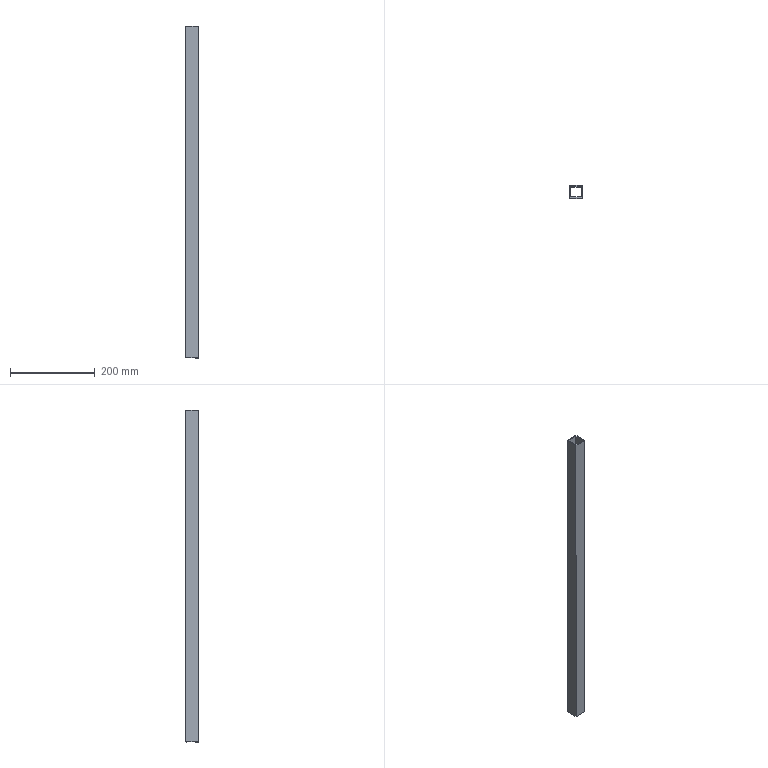Part | SolidWorks | features Extrusion 1 | 1 solid | 10 faces | box 30 x 30 x 784 mm | volume 254016 mm3 | plane 10
STEP:
#1=CARTESIAN_POINT('',(-16.115,15.846,784.));
#2=VERTEX_POINT('',#1);
#3=CARTESIAN_POINT('',(-16.115,-14.154,784.));
#4=VERTEX_POINT('',#3);
#5=CARTESIAN_POINT('',(-16.115,-14.154,784.));
#6=DIRECTION('',(0.,-1.,0.));
#7=VECTOR('',#6,1000.);
#8=LINE('',#5,#7);
#9=EDGE_CURVE('',#2,#4,#8,.T.);
#10=ORIENTED_EDGE('',*,*,#9,.T.);
#11=CARTESIAN_POINT('',(13.885,-14.154,784.));
#12=VERTEX_POINT('',#11);
#13=CARTESIAN_POINT('',(13.885,-14.154,784.));
#14=DIRECTION('',(1.,0.,0.));
#15=VECTOR('',#14,1000.);
#16=LINE('',#13,#15);
#17=EDGE_CURVE('',#4,#12,#16,.T.);
#18=ORIENTED_EDGE('',*,*,#17,.T.);
#19=CARTESIAN_POINT('',(13.885,15.846,784.));
#20=VERTEX_POINT('',#19);
#21=CARTESIAN_POINT('',(13.885,15.846,784.));
#22=DIRECTION('',(0.,1.,0.));
#23=VECTOR('',#22,1000.);
#24=LINE('',#21,#23);
#25=EDGE_CURVE('',#12,#20,#24,.T.);
#26=ORIENTED_EDGE('',*,*,#25,.T.);
#27=CARTESIAN_POINT('',(-16.115,15.846,784.));
#28=DIRECTION('',(-1.,0.,0.));
#29=VECTOR('',#28,1000.);
#30=LINE('',#27,#29);
#31=EDGE_CURVE('',#20,#2,#30,.T.);
#32=ORIENTED_EDGE('',*,*,#31,.T.);
#33=EDGE_LOOP('',(#10,#18,#26,#32));
#34=FACE_OUTER_BOUND('',#33,.T.);
#35=CARTESIAN_POINT('',(-13.115,12.846,784.));
#36=VERTEX_POINT('',#35);
#37=CARTESIAN_POINT('',(-13.115,-11.154,784.));
#38=VERTEX_POINT('',#37);
#39=CARTESIAN_POINT('',(-13.115,-11.154,784.));
#40=DIRECTION('',(0.,-1.,0.));
#41=VECTOR('',#40,1000.);
#42=LINE('',#39,#41);
#43=EDGE_CURVE('',#36,#38,#42,.T.);
#44=ORIENTED_EDGE('',*,*,#43,.F.);
#45=CARTESIAN_POINT('',(10.885,12.846,784.));
#46=VERTEX_POINT('',#45);
#47=CARTESIAN_POINT('',(-13.115,12.846,784.));
#48=DIRECTION('',(-1.,0.,0.));
#49=VECTOR('',#48,1000.);
#50=LINE('',#47,#49);
#51=EDGE_CURVE('',#46,#36,#50,.T.);
#52=ORIENTED_EDGE('',*,*,#51,.F.);
#53=CARTESIAN_POINT('',(10.885,-11.154,784.));
#54=VERTEX_POINT('',#53);
#55=CARTESIAN_POINT('',(10.885,12.846,784.));
#56=DIRECTION('',(0.,1.,0.));
#57=VECTOR('',#56,1000.);
#58=LINE('',#55,#57);
#59=EDGE_CURVE('',#54,#46,#58,.T.);
#60=ORIENTED_EDGE('',*,*,#59,.F.);
#61=CARTESIAN_POINT('',(10.885,-11.154,784.));
#62=DIRECTION('',(1.,0.,0.));
#63=VECTOR('',#62,1000.);
#64=LINE('',#61,#63);
#65=EDGE_CURVE('',#38,#54,#64,.T.);
#66=ORIENTED_EDGE('',*,*,#65,.F.);
#67=EDGE_LOOP('',(#44,#52,#60,#66));
#68=FACE_BOUND('',#67,.T.);
#69=CARTESIAN_POINT('',(-0.000000003,0.000000004,784.));
#70=DIRECTION('',(0.,0.,-1.));
#71=DIRECTION('',(-1.,0.,0.));
#72=AXIS2_PLACEMENT_3D('',#69,#70,#71);
#73=PLANE('',#72);
#74=ADVANCED_FACE('',(#34,#68),#73,.F.);
#75=CARTESIAN_POINT('',(-16.115,15.846,0.000000013));
#76=VERTEX_POINT('',#75);
#77=CARTESIAN_POINT('',(-16.115,-14.154,0.000000013));
#78=VERTEX_POINT('',#77);
#79=CARTESIAN_POINT('',(-16.115,-14.154,0.000000013));
#80=DIRECTION('',(0.,-1.,0.));
#81=VECTOR('',#80,1000.);
#82=LINE('',#79,#81);
#83=EDGE_CURVE('',#76,#78,#82,.T.);
#84=ORIENTED_EDGE('',*,*,#83,.F.);
#85=CARTESIAN_POINT('',(13.885,15.846,0.000000013));
#86=VERTEX_POINT('',#85);
#87=CARTESIAN_POINT('',(-16.115,15.846,0.000000013));
#88=DIRECTION('',(-1.,0.,0.));
#89=VECTOR('',#88,1000.);
#90=LINE('',#87,#89);
#91=EDGE_CURVE('',#86,#76,#90,.T.);
#92=ORIENTED_EDGE('',*,*,#91,.F.);
#93=CARTESIAN_POINT('',(13.885,-14.154,0.000000013));
#94=VERTEX_POINT('',#93);
#95=CARTESIAN_POINT('',(13.885,15.846,0.000000013));
#96=DIRECTION('',(0.,1.,0.));
#97=VECTOR('',#96,1000.);
#98=LINE('',#95,#97);
#99=EDGE_CURVE('',#94,#86,#98,.T.);
#100=ORIENTED_EDGE('',*,*,#99,.F.);
#101=CARTESIAN_POINT('',(13.885,-14.154,0.000000013));
#102=DIRECTION('',(1.,0.,0.));
#103=VECTOR('',#102,1000.);
#104=LINE('',#101,#103);
#105=EDGE_CURVE('',#78,#94,#104,.T.);
#106=ORIENTED_EDGE('',*,*,#105,.F.);
#107=EDGE_LOOP('',(#84,#92,#100,#106));
#108=FACE_OUTER_BOUND('',#107,.T.);
#109=CARTESIAN_POINT('',(10.885,12.846,0.000000013));
#110=VERTEX_POINT('',#109);
#111=CARTESIAN_POINT('',(-13.115,12.846,0.000000013));
#112=VERTEX_POINT('',#111);
#113=CARTESIAN_POINT('',(-13.115,12.846,0.000000013));
#114=DIRECTION('',(-1.,0.,0.));
#115=VECTOR('',#114,1000.);
#116=LINE('',#113,#115);
#117=EDGE_CURVE('',#110,#112,#116,.T.);
#118=ORIENTED_EDGE('',*,*,#117,.T.);
#119=CARTESIAN_POINT('',(-13.115,-11.154,0.000000013));
#120=VERTEX_POINT('',#119);
#121=CARTESIAN_POINT('',(-13.115,-11.154,0.000000013));
#122=DIRECTION('',(0.,-1.,0.));
#123=VECTOR('',#122,1000.);
#124=LINE('',#121,#123);
#125=EDGE_CURVE('',#112,#120,#124,.T.);
#126=ORIENTED_EDGE('',*,*,#125,.T.);
#127=CARTESIAN_POINT('',(10.885,-11.154,0.000000013));
#128=VERTEX_POINT('',#127);
#129=CARTESIAN_POINT('',(10.885,-11.154,0.000000013));
#130=DIRECTION('',(1.,0.,0.));
#131=VECTOR('',#130,1000.);
#132=LINE('',#129,#131);
#133=EDGE_CURVE('',#120,#128,#132,.T.);
#134=ORIENTED_EDGE('',*,*,#133,.T.);
#135=CARTESIAN_POINT('',(10.885,12.846,0.000000013));
#136=DIRECTION('',(0.,1.,0.));
#137=VECTOR('',#136,1000.);
#138=LINE('',#135,#137);
#139=EDGE_CURVE('',#128,#110,#138,.T.);
#140=ORIENTED_EDGE('',*,*,#139,.T.);
#141=EDGE_LOOP('',(#118,#126,#134,#140));
#142=FACE_BOUND('',#141,.T.);
#143=CARTESIAN_POINT('',(-0.000000003,0.000000004,0.000000013));
#144=DIRECTION('',(0.,0.,-1.));
#145=DIRECTION('',(-1.,0.,0.));
#146=AXIS2_PLACEMENT_3D('',#143,#144,#145);
#147=PLANE('',#146);
#148=ADVANCED_FACE('',(#108,#142),#147,.T.);
#149=ORIENTED_EDGE('',*,*,#83,.T.);
#150=CARTESIAN_POINT('',(-16.115,-14.154,784.));
#151=DIRECTION('',(0.,0.,-1.));
#152=VECTOR('',#151,1000.);
#153=LINE('',#150,#152);
#154=EDGE_CURVE('',#4,#78,#153,.T.);
#155=ORIENTED_EDGE('',*,*,#154,.F.);
#156=ORIENTED_EDGE('',*,*,#9,.F.);
#157=CARTESIAN_POINT('',(-16.115,15.846,784.));
#158=DIRECTION('',(0.,0.,-1.));
#159=VECTOR('',#158,1000.);
#160=LINE('',#157,#159);
#161=EDGE_CURVE('',#2,#76,#160,.T.);
#162=ORIENTED_EDGE('',*,*,#161,.T.);
#163=EDGE_LOOP('',(#149,#155,#156,#162));
#164=FACE_OUTER_BOUND('',#163,.T.);
#165=CARTESIAN_POINT('',(-16.115,-14.154,784.));
#166=DIRECTION('',(1.,0.,0.));
#167=DIRECTION('',(0.,0.,-1.));
#168=AXIS2_PLACEMENT_3D('',#165,#166,#167);
#169=PLANE('',#168);
#170=ADVANCED_FACE('',(#164),#169,.F.);
#171=ORIENTED_EDGE('',*,*,#105,.T.);
#172=CARTESIAN_POINT('',(13.885,-14.154,784.));
#173=DIRECTION('',(0.,0.,-1.));
#174=VECTOR('',#173,1000.);
#175=LINE('',#172,#174);
#176=EDGE_CURVE('',#12,#94,#175,.T.);
#177=ORIENTED_EDGE('',*,*,#176,.F.);
#178=ORIENTED_EDGE('',*,*,#17,.F.);
#179=ORIENTED_EDGE('',*,*,#154,.T.);
#180=EDGE_LOOP('',(#171,#177,#178,#179));
#181=FACE_OUTER_BOUND('',#180,.T.);
#182=CARTESIAN_POINT('',(13.885,-14.154,784.));
#183=DIRECTION('',(0.,1.,0.));
#184=DIRECTION('',(-1.,0.,0.));
#185=AXIS2_PLACEMENT_3D('',#182,#183,#184);
#186=PLANE('',#185);
#187=ADVANCED_FACE('',(#181),#186,.F.);
#188=ORIENTED_EDGE('',*,*,#99,.T.);
#189=CARTESIAN_POINT('',(13.885,15.846,784.));
#190=DIRECTION('',(0.,0.,-1.));
#191=VECTOR('',#190,1000.);
#192=LINE('',#189,#191);
#193=EDGE_CURVE('',#20,#86,#192,.T.);
#194=ORIENTED_EDGE('',*,*,#193,.F.);
#195=ORIENTED_EDGE('',*,*,#25,.F.);
#196=ORIENTED_EDGE('',*,*,#176,.T.);
#197=EDGE_LOOP('',(#188,#194,#195,#196));
#198=FACE_OUTER_BOUND('',#197,.T.);
#199=CARTESIAN_POINT('',(13.885,15.846,784.));
#200=DIRECTION('',(-1.,0.,0.));
#201=DIRECTION('',(0.,-1.,0.));
#202=AXIS2_PLACEMENT_3D('',#199,#200,#201);
#203=PLANE('',#202);
#204=ADVANCED_FACE('',(#198),#203,.F.);
#205=ORIENTED_EDGE('',*,*,#91,.T.);
#206=ORIENTED_EDGE('',*,*,#161,.F.);
#207=ORIENTED_EDGE('',*,*,#31,.F.);
#208=ORIENTED_EDGE('',*,*,#193,.T.);
#209=EDGE_LOOP('',(#205,#206,#207,#208));
#210=FACE_OUTER_BOUND('',#209,.T.);
#211=CARTESIAN_POINT('',(-16.115,15.846,784.));
#212=DIRECTION('',(0.,-1.,0.));
#213=DIRECTION('',(0.,0.,-1.));
#214=AXIS2_PLACEMENT_3D('',#211,#212,#213);
#215=PLANE('',#214);
#216=ADVANCED_FACE('',(#210),#215,.F.);
#217=ORIENTED_EDGE('',*,*,#125,.F.);
#218=CARTESIAN_POINT('',(-13.115,12.846,784.));
#219=DIRECTION('',(0.,0.,-1.));
#220=VECTOR('',#219,1000.);
#221=LINE('',#218,#220);
#222=EDGE_CURVE('',#36,#112,#221,.T.);
#223=ORIENTED_EDGE('',*,*,#222,.F.);
#224=ORIENTED_EDGE('',*,*,#43,.T.);
#225=CARTESIAN_POINT('',(-13.115,-11.154,784.));
#226=DIRECTION('',(0.,0.,-1.));
#227=VECTOR('',#226,1000.);
#228=LINE('',#225,#227);
#229=EDGE_CURVE('',#38,#120,#228,.T.);
#230=ORIENTED_EDGE('',*,*,#229,.T.);
#231=EDGE_LOOP('',(#217,#223,#224,#230));
#232=FACE_OUTER_BOUND('',#231,.T.);
#233=CARTESIAN_POINT('',(-13.115,-11.154,784.));
#234=DIRECTION('',(1.,0.,0.));
#235=DIRECTION('',(0.,1.,0.));
#236=AXIS2_PLACEMENT_3D('',#233,#234,#235);
#237=PLANE('',#236);
#238=ADVANCED_FACE('',(#232),#237,.T.);
#239=ORIENTED_EDGE('',*,*,#133,.F.);
#240=ORIENTED_EDGE('',*,*,#229,.F.);
#241=ORIENTED_EDGE('',*,*,#65,.T.);
#242=CARTESIAN_POINT('',(10.885,-11.154,784.));
#243=DIRECTION('',(0.,0.,-1.));
#244=VECTOR('',#243,1000.);
#245=LINE('',#242,#244);
#246=EDGE_CURVE('',#54,#128,#245,.T.);
#247=ORIENTED_EDGE('',*,*,#246,.T.);
#248=EDGE_LOOP('',(#239,#240,#241,#247));
#249=FACE_OUTER_BOUND('',#248,.T.);
#250=CARTESIAN_POINT('',(10.885,-11.154,784.));
#251=DIRECTION('',(0.,1.,0.));
#252=DIRECTION('',(-1.,0.,0.));
#253=AXIS2_PLACEMENT_3D('',#250,#251,#252);
#254=PLANE('',#253);
#255=ADVANCED_FACE('',(#249),#254,.T.);
#256=ORIENTED_EDGE('',*,*,#139,.F.);
#257=ORIENTED_EDGE('',*,*,#246,.F.);
#258=ORIENTED_EDGE('',*,*,#59,.T.);
#259=CARTESIAN_POINT('',(10.885,12.846,784.));
#260=DIRECTION('',(0.,0.,-1.));
#261=VECTOR('',#260,1000.);
#262=LINE('',#259,#261);
#263=EDGE_CURVE('',#46,#110,#262,.T.);
#264=ORIENTED_EDGE('',*,*,#263,.T.);
#265=EDGE_LOOP('',(#256,#257,#258,#264));
#266=FACE_OUTER_BOUND('',#265,.T.);
#267=CARTESIAN_POINT('',(10.885,12.846,784.));
#268=DIRECTION('',(-1.,0.,0.));
#269=DIRECTION('',(0.,-1.,0.));
#270=AXIS2_PLACEMENT_3D('',#267,#268,#269);
#271=PLANE('',#270);
#272=ADVANCED_FACE('',(#266),#271,.T.);
#273=ORIENTED_EDGE('',*,*,#117,.F.);
#274=ORIENTED_EDGE('',*,*,#263,.F.);
#275=ORIENTED_EDGE('',*,*,#51,.T.);
#276=ORIENTED_EDGE('',*,*,#222,.T.);
#277=EDGE_LOOP('',(#273,#274,#275,#276));
#278=FACE_OUTER_BOUND('',#277,.T.);
#279=CARTESIAN_POINT('',(-13.115,12.846,784.));
#280=DIRECTION('',(0.,-1.,0.));
#281=DIRECTION('',(0.,0.,-1.));
#282=AXIS2_PLACEMENT_3D('',#279,#280,#281);
#283=PLANE('',#282);
#284=ADVANCED_FACE('',(#278),#283,.T.);
#285=CLOSED_SHELL('',(#74,#148,#170,#187,#204,#216,#238,#255,#272,#284));
#286=MANIFOLD_SOLID_BREP('',#285);
#287=CARTESIAN_POINT('',(0.,0.,0.));
#288=DIRECTION('',(0.,0.,1.));
#289=DIRECTION('',(1.,0.,0.));
#290=AXIS2_PLACEMENT_3D('',#287,#288,#289);
#291=(LENGTH_UNIT()NAMED_UNIT(*)SI_UNIT(.MILLI.,.METRE.));
#292=UNCERTAINTY_MEASURE_WITH_UNIT(LENGTH_MEASURE(0.00001),#291,'','');
#293=(NAMED_UNIT(*)PLANE_ANGLE_UNIT()SI_UNIT($,.RADIAN.));
#294=(NAMED_UNIT(*)SI_UNIT($,.STERADIAN.)SOLID_ANGLE_UNIT());
#295=(GEOMETRIC_REPRESENTATION_CONTEXT(3)GLOBAL_UNCERTAINTY_ASSIGNED_CONTEXT((#292))GLOBAL_UNIT_ASSIGNED_CONTEXT((#291,#293,#294))REPRESENTATION_CONTEXT('',''));
#296=ADVANCED_BREP_SHAPE_REPRESENTATION('',(#286,#290),#295);